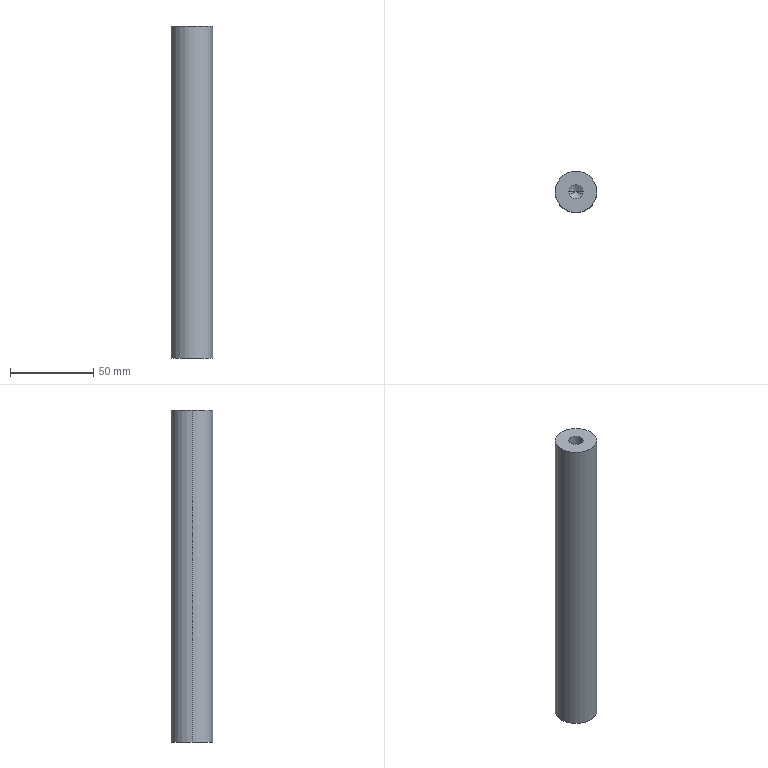Part | STEP file | B1-004 | 1 solid | 12 faces | box 25 x 25 x 200 mm | volume 96489 mm3 | cylinder 6 | cone 4 | plane 2 | commonest cylinder face diameters 8.5 x4 25 x2
STEP:
#1=CARTESIAN_POINT('',(0.,0.,0.));
#2=DIRECTION('',(0.,0.,1.));
#3=DIRECTION('',(1.,0.,0.));
#4=AXIS2_PLACEMENT_3D('',#1,#2,#3);
#5=CARTESIAN_POINT('',(4.25,0.,86.));
#6=VERTEX_POINT('',#5);
#7=CARTESIAN_POINT('',(4.25,0.,100.));
#8=VERTEX_POINT('',#7);
#9=CARTESIAN_POINT('',(4.25,0.,100.));
#10=DIRECTION('',(0.,0.,1.));
#11=VECTOR('',#10,1.);
#12=LINE('',#9,#11);
#13=CARTESIAN_POINT('',(0.,0.,100.));
#14=DIRECTION('',(0.,0.,1.));
#15=DIRECTION('',(1.,0.,0.));
#16=AXIS2_PLACEMENT_3D('',#13,#14,#15);
#17=CYLINDRICAL_SURFACE('',#16,4.25);
#18=CARTESIAN_POINT('',(6.283,0.));
#19=DIRECTION('',(0.,1.));
#20=VECTOR('',#19,1.);
#21=LINE('',#18,#20);
#22=(GEOMETRIC_REPRESENTATION_CONTEXT(2)PARAMETRIC_REPRESENTATION_CONTEXT()REPRESENTATION_CONTEXT('',''));
#23=DEFINITIONAL_REPRESENTATION('',(#21),#22);
#24=PCURVE('',#17,#23);
#25=CARTESIAN_POINT('',(0.,0.,100.));
#26=DIRECTION('',(0.,0.,1.));
#27=DIRECTION('',(1.,0.,0.));
#28=AXIS2_PLACEMENT_3D('',#25,#26,#27);
#29=CYLINDRICAL_SURFACE('',#28,4.25);
#30=CARTESIAN_POINT('',(0.,0.));
#31=DIRECTION('',(0.,1.));
#32=VECTOR('',#31,1.);
#33=LINE('',#30,#32);
#34=(GEOMETRIC_REPRESENTATION_CONTEXT(2)PARAMETRIC_REPRESENTATION_CONTEXT()REPRESENTATION_CONTEXT('',''));
#35=DEFINITIONAL_REPRESENTATION('',(#33),#34);
#36=PCURVE('',#29,#35);
#37=SURFACE_CURVE('',#12,(#24,#36),.PCURVE_S1.);
#38=EDGE_CURVE('',#6,#8,#37,.T.);
#39=ORIENTED_EDGE('',*,*,#38,.T.);
#40=CARTESIAN_POINT('',(-4.25,0.,100.));
#41=VERTEX_POINT('',#40);
#42=CARTESIAN_POINT('',(0.,0.,100.));
#43=DIRECTION('',(0.,0.,1.));
#44=DIRECTION('',(1.,0.,0.));
#45=AXIS2_PLACEMENT_3D('',#42,#43,#44);
#46=CIRCLE('',#45,4.25);
#47=CARTESIAN_POINT('',(0.,0.));
#48=DIRECTION('',(1.,0.));
#49=VECTOR('',#48,1.);
#50=LINE('',#47,#49);
#51=(GEOMETRIC_REPRESENTATION_CONTEXT(2)PARAMETRIC_REPRESENTATION_CONTEXT()REPRESENTATION_CONTEXT('',''));
#52=DEFINITIONAL_REPRESENTATION('',(#50),#51);
#53=PCURVE('',#17,#52);
#54=CARTESIAN_POINT('',(0.,0.,100.));
#55=DIRECTION('',(0.,0.,1.));
#56=DIRECTION('',(1.,0.,0.));
#57=AXIS2_PLACEMENT_3D('',#54,#55,#56);
#58=PLANE('',#57);
#59=CARTESIAN_POINT('',(0.,0.));
#60=DIRECTION('',(1.,0.));
#61=AXIS2_PLACEMENT_2D('',#59,#60);
#62=CIRCLE('',#61,4.25);
#63=(GEOMETRIC_REPRESENTATION_CONTEXT(2)PARAMETRIC_REPRESENTATION_CONTEXT()REPRESENTATION_CONTEXT('',''));
#64=DEFINITIONAL_REPRESENTATION('',(#62),#63);
#65=PCURVE('',#58,#64);
#66=SURFACE_CURVE('',#46,(#53,#65),.PCURVE_S1.);
#67=EDGE_CURVE('',#41,#8,#66,.T.);
#68=ORIENTED_EDGE('',*,*,#67,.F.);
#69=CARTESIAN_POINT('',(-4.25,0.,86.));
#70=VERTEX_POINT('',#69);
#71=CARTESIAN_POINT('',(-4.25,0.,100.));
#72=DIRECTION('',(0.,0.,1.));
#73=VECTOR('',#72,1.);
#74=LINE('',#71,#73);
#75=CARTESIAN_POINT('',(3.142,0.));
#76=DIRECTION('',(0.,1.));
#77=VECTOR('',#76,1.);
#78=LINE('',#75,#77);
#79=(GEOMETRIC_REPRESENTATION_CONTEXT(2)PARAMETRIC_REPRESENTATION_CONTEXT()REPRESENTATION_CONTEXT('',''));
#80=DEFINITIONAL_REPRESENTATION('',(#78),#79);
#81=PCURVE('',#17,#80);
#82=CARTESIAN_POINT('',(3.142,0.));
#83=DIRECTION('',(0.,1.));
#84=VECTOR('',#83,1.);
#85=LINE('',#82,#84);
#86=(GEOMETRIC_REPRESENTATION_CONTEXT(2)PARAMETRIC_REPRESENTATION_CONTEXT()REPRESENTATION_CONTEXT('',''));
#87=DEFINITIONAL_REPRESENTATION('',(#85),#86);
#88=PCURVE('',#29,#87);
#89=SURFACE_CURVE('',#74,(#81,#88),.PCURVE_S1.);
#90=EDGE_CURVE('',#70,#41,#89,.T.);
#91=ORIENTED_EDGE('',*,*,#90,.F.);
#92=CARTESIAN_POINT('',(0.,0.,86.));
#93=DIRECTION('',(0.,0.,1.));
#94=DIRECTION('',(1.,0.,0.));
#95=AXIS2_PLACEMENT_3D('',#92,#93,#94);
#96=CIRCLE('',#95,4.25);
#97=CARTESIAN_POINT('',(0.,-14.));
#98=DIRECTION('',(1.,0.));
#99=VECTOR('',#98,1.);
#100=LINE('',#97,#99);
#101=(GEOMETRIC_REPRESENTATION_CONTEXT(2)PARAMETRIC_REPRESENTATION_CONTEXT()REPRESENTATION_CONTEXT('',''));
#102=DEFINITIONAL_REPRESENTATION('',(#100),#101);
#103=PCURVE('',#17,#102);
#104=CARTESIAN_POINT('',(0.,0.,86.));
#105=DIRECTION('',(0.,0.,1.));
#106=DIRECTION('',(1.,0.,0.));
#107=AXIS2_PLACEMENT_3D('',#104,#105,#106);
#108=CONICAL_SURFACE('',#107,4.25,1.03);
#109=CARTESIAN_POINT('',(0.,0.));
#110=DIRECTION('',(1.,0.));
#111=VECTOR('',#110,1.);
#112=LINE('',#109,#111);
#113=(GEOMETRIC_REPRESENTATION_CONTEXT(2)PARAMETRIC_REPRESENTATION_CONTEXT()REPRESENTATION_CONTEXT('',''));
#114=DEFINITIONAL_REPRESENTATION('',(#112),#113);
#115=PCURVE('',#108,#114);
#116=SURFACE_CURVE('',#96,(#103,#115),.PCURVE_S1.);
#117=EDGE_CURVE('',#70,#6,#116,.T.);
#118=ORIENTED_EDGE('',*,*,#117,.T.);
#119=EDGE_LOOP('',(#39,#68,#91,#118));
#120=FACE_BOUND('',#119,.F.);
#121=ADVANCED_FACE('',(#120),#17,.F.);
#122=ORIENTED_EDGE('',*,*,#117,.F.);
#123=CARTESIAN_POINT('',(0.,0.,83.446));
#124=VERTEX_POINT('',#123);
#125=CARTESIAN_POINT('',(-4.25,0.,86.));
#126=DIRECTION('',(-0.8572,0.,0.515));
#127=VECTOR('',#126,1.);
#128=LINE('',#125,#127);
#129=CARTESIAN_POINT('',(3.142,-2.554));
#130=CARTESIAN_POINT('',(3.142,-2.515));
#131=CARTESIAN_POINT('',(3.142,-2.438));
#132=CARTESIAN_POINT('',(3.142,-2.322));
#133=CARTESIAN_POINT('',(3.142,-2.205));
#134=CARTESIAN_POINT('',(3.142,-2.089));
#135=CARTESIAN_POINT('',(3.142,-1.973));
#136=CARTESIAN_POINT('',(3.142,-1.857));
#137=CARTESIAN_POINT('',(3.142,-1.741));
#138=CARTESIAN_POINT('',(3.142,-1.625));
#139=CARTESIAN_POINT('',(3.142,-1.509));
#140=CARTESIAN_POINT('',(3.142,-1.393));
#141=CARTESIAN_POINT('',(3.142,-1.277));
#142=CARTESIAN_POINT('',(3.142,-1.161));
#143=CARTESIAN_POINT('',(3.142,-1.045));
#144=CARTESIAN_POINT('',(3.142,-0.9286));
#145=CARTESIAN_POINT('',(3.142,-0.8125));
#146=CARTESIAN_POINT('',(3.142,-0.6965));
#147=CARTESIAN_POINT('',(3.142,-0.5804));
#148=CARTESIAN_POINT('',(3.142,-0.4643));
#149=CARTESIAN_POINT('',(3.142,-0.3482));
#150=CARTESIAN_POINT('',(3.142,-0.2322));
#151=CARTESIAN_POINT('',(3.142,-0.1161));
#152=CARTESIAN_POINT('',(3.142,-0.03869));
#153=CARTESIAN_POINT('',(3.142,0.));
#154=B_SPLINE_CURVE_WITH_KNOTS('',3,(#129,#130,#131,#132,#133,#134,#135,#136,#137,#138,#139,#140,#141,#142,#143,#144,#145,#146,#147,#148,#149,#150,#151,#152,#153),.UNSPECIFIED.,.F.,.F.,(4,1,1,1,1,1,1,1,1,1,1,1,1,1,1,1,1,1,1,1,1,1,4),(-4.958,-4.733,-4.507,-4.282,-4.057,-3.831,-3.606,-3.381,-3.155,-2.93,-2.704,-2.479,-2.254,-2.028,-1.803,-1.578,-1.352,-1.127,-0.9015,-0.6761,-0.4507,-0.2254,0.),.UNSPECIFIED.);
#155=(GEOMETRIC_REPRESENTATION_CONTEXT(2)PARAMETRIC_REPRESENTATION_CONTEXT()REPRESENTATION_CONTEXT('',''));
#156=DEFINITIONAL_REPRESENTATION('',(#154),#155);
#157=PCURVE('',#108,#156);
#158=CARTESIAN_POINT('',(0.,0.,86.));
#159=DIRECTION('',(0.,0.,1.));
#160=DIRECTION('',(1.,0.,0.));
#161=AXIS2_PLACEMENT_3D('',#158,#159,#160);
#162=CONICAL_SURFACE('',#161,4.25,1.03);
#163=CARTESIAN_POINT('',(3.142,-2.554));
#164=CARTESIAN_POINT('',(3.142,-2.515));
#165=CARTESIAN_POINT('',(3.142,-2.438));
#166=CARTESIAN_POINT('',(3.142,-2.322));
#167=CARTESIAN_POINT('',(3.142,-2.205));
#168=CARTESIAN_POINT('',(3.142,-2.089));
#169=CARTESIAN_POINT('',(3.142,-1.973));
#170=CARTESIAN_POINT('',(3.142,-1.857));
#171=CARTESIAN_POINT('',(3.142,-1.741));
#172=CARTESIAN_POINT('',(3.142,-1.625));
#173=CARTESIAN_POINT('',(3.142,-1.509));
#174=CARTESIAN_POINT('',(3.142,-1.393));
#175=CARTESIAN_POINT('',(3.142,-1.277));
#176=CARTESIAN_POINT('',(3.142,-1.161));
#177=CARTESIAN_POINT('',(3.142,-1.045));
#178=CARTESIAN_POINT('',(3.142,-0.9286));
#179=CARTESIAN_POINT('',(3.142,-0.8125));
#180=CARTESIAN_POINT('',(3.142,-0.6965));
#181=CARTESIAN_POINT('',(3.142,-0.5804));
#182=CARTESIAN_POINT('',(3.142,-0.4643));
#183=CARTESIAN_POINT('',(3.142,-0.3482));
#184=CARTESIAN_POINT('',(3.142,-0.2322));
#185=CARTESIAN_POINT('',(3.142,-0.1161));
#186=CARTESIAN_POINT('',(3.142,-0.03869));
#187=CARTESIAN_POINT('',(3.142,0.));
#188=B_SPLINE_CURVE_WITH_KNOTS('',3,(#163,#164,#165,#166,#167,#168,#169,#170,#171,#172,#173,#174,#175,#176,#177,#178,#179,#180,#181,#182,#183,#184,#185,#186,#187),.UNSPECIFIED.,.F.,.F.,(4,1,1,1,1,1,1,1,1,1,1,1,1,1,1,1,1,1,1,1,1,1,4),(-4.958,-4.733,-4.507,-4.282,-4.057,-3.831,-3.606,-3.381,-3.155,-2.93,-2.704,-2.479,-2.254,-2.028,-1.803,-1.578,-1.352,-1.127,-0.9015,-0.6761,-0.4507,-0.2254,0.),.UNSPECIFIED.);
#189=(GEOMETRIC_REPRESENTATION_CONTEXT(2)PARAMETRIC_REPRESENTATION_CONTEXT()REPRESENTATION_CONTEXT('',''));
#190=DEFINITIONAL_REPRESENTATION('',(#188),#189);
#191=PCURVE('',#162,#190);
#192=SURFACE_CURVE('',#128,(#157,#191),.PCURVE_S1.);
#193=EDGE_CURVE('',#124,#70,#192,.T.);
#194=ORIENTED_EDGE('',*,*,#193,.F.);
#195=CARTESIAN_POINT('',(4.25,0.,86.));
#196=DIRECTION('',(0.8572,0.,0.515));
#197=VECTOR('',#196,1.);
#198=LINE('',#195,#197);
#199=CARTESIAN_POINT('',(6.283,0.));
#200=DIRECTION('',(0.,1.));
#201=VECTOR('',#200,1.);
#202=LINE('',#199,#201);
#203=(GEOMETRIC_REPRESENTATION_CONTEXT(2)PARAMETRIC_REPRESENTATION_CONTEXT()REPRESENTATION_CONTEXT('',''));
#204=DEFINITIONAL_REPRESENTATION('',(#202),#203);
#205=PCURVE('',#108,#204);
#206=CARTESIAN_POINT('',(0.,0.));
#207=DIRECTION('',(0.,1.));
#208=VECTOR('',#207,1.);
#209=LINE('',#206,#208);
#210=(GEOMETRIC_REPRESENTATION_CONTEXT(2)PARAMETRIC_REPRESENTATION_CONTEXT()REPRESENTATION_CONTEXT('',''));
#211=DEFINITIONAL_REPRESENTATION('',(#209),#210);
#212=PCURVE('',#162,#211);
#213=SURFACE_CURVE('',#198,(#205,#212),.PCURVE_S1.);
#214=EDGE_CURVE('',#124,#6,#213,.T.);
#215=ORIENTED_EDGE('',*,*,#214,.T.);
#216=EDGE_LOOP('',(#122,#194,#215));
#217=FACE_BOUND('',#216,.F.);
#218=ADVANCED_FACE('',(#217),#108,.F.);
#219=CARTESIAN_POINT('',(-4.25,0.,-86.));
#220=VERTEX_POINT('',#219);
#221=CARTESIAN_POINT('',(-4.25,0.,-100.));
#222=VERTEX_POINT('',#221);
#223=CARTESIAN_POINT('',(-4.25,0.,-100.));
#224=DIRECTION('',(0.,0.,-1.));
#225=VECTOR('',#224,1.);
#226=LINE('',#223,#225);
#227=CARTESIAN_POINT('',(0.,0.,-100.));
#228=DIRECTION('',(0.,0.,-1.));
#229=DIRECTION('',(-1.,0.,0.));
#230=AXIS2_PLACEMENT_3D('',#227,#228,#229);
#231=CYLINDRICAL_SURFACE('',#230,4.25);
#232=CARTESIAN_POINT('',(6.283,0.));
#233=DIRECTION('',(0.,1.));
#234=VECTOR('',#233,1.);
#235=LINE('',#232,#234);
#236=(GEOMETRIC_REPRESENTATION_CONTEXT(2)PARAMETRIC_REPRESENTATION_CONTEXT()REPRESENTATION_CONTEXT('',''));
#237=DEFINITIONAL_REPRESENTATION('',(#235),#236);
#238=PCURVE('',#231,#237);
#239=CARTESIAN_POINT('',(0.,0.,-100.));
#240=DIRECTION('',(0.,0.,-1.));
#241=DIRECTION('',(-1.,0.,0.));
#242=AXIS2_PLACEMENT_3D('',#239,#240,#241);
#243=CYLINDRICAL_SURFACE('',#242,4.25);
#244=CARTESIAN_POINT('',(0.,0.));
#245=DIRECTION('',(0.,1.));
#246=VECTOR('',#245,1.);
#247=LINE('',#244,#246);
#248=(GEOMETRIC_REPRESENTATION_CONTEXT(2)PARAMETRIC_REPRESENTATION_CONTEXT()REPRESENTATION_CONTEXT('',''));
#249=DEFINITIONAL_REPRESENTATION('',(#247),#248);
#250=PCURVE('',#243,#249);
#251=SURFACE_CURVE('',#226,(#238,#250),.PCURVE_S1.);
#252=EDGE_CURVE('',#220,#222,#251,.T.);
#253=ORIENTED_EDGE('',*,*,#252,.T.);
#254=CARTESIAN_POINT('',(4.25,0.,-100.));
#255=VERTEX_POINT('',#254);
#256=CARTESIAN_POINT('',(0.,0.,-100.));
#257=DIRECTION('',(0.,0.,-1.));
#258=DIRECTION('',(-1.,0.,0.));
#259=AXIS2_PLACEMENT_3D('',#256,#257,#258);
#260=CIRCLE('',#259,4.25);
#261=CARTESIAN_POINT('',(0.,0.));
#262=DIRECTION('',(1.,0.));
#263=VECTOR('',#262,1.);
#264=LINE('',#261,#263);
#265=(GEOMETRIC_REPRESENTATION_CONTEXT(2)PARAMETRIC_REPRESENTATION_CONTEXT()REPRESENTATION_CONTEXT('',''));
#266=DEFINITIONAL_REPRESENTATION('',(#264),#265);
#267=PCURVE('',#231,#266);
#268=CARTESIAN_POINT('',(0.,0.,-100.));
#269=DIRECTION('',(0.,0.,1.));
#270=DIRECTION('',(1.,0.,0.));
#271=AXIS2_PLACEMENT_3D('',#268,#269,#270);
#272=PLANE('',#271);
#273=CARTESIAN_POINT('',(-4.25,0.));
#274=CARTESIAN_POINT('',(-4.25,7.361));
#275=CARTESIAN_POINT('',(2.125,3.681));
#276=CARTESIAN_POINT('',(8.5,0.));
#277=CARTESIAN_POINT('',(2.125,-3.681));
#278=CARTESIAN_POINT('',(-4.25,-7.361));
#279=CARTESIAN_POINT('',(-4.25,0.));
#280=(BOUNDED_CURVE()B_SPLINE_CURVE(2,(#273,#274,#275,#276,#277,#278,#279),.UNSPECIFIED.,.T.,.F.)B_SPLINE_CURVE_WITH_KNOTS((1,2,2,2,2,1),(-2.094,0.,2.094,4.189,6.283,8.378),.UNSPECIFIED.)CURVE()GEOMETRIC_REPRESENTATION_ITEM()RATIONAL_B_SPLINE_CURVE((1.,0.5,1.,0.5,1.,0.5,1.))REPRESENTATION_ITEM(''));
#281=(GEOMETRIC_REPRESENTATION_CONTEXT(2)PARAMETRIC_REPRESENTATION_CONTEXT()REPRESENTATION_CONTEXT('',''));
#282=DEFINITIONAL_REPRESENTATION('',(#280),#281);
#283=PCURVE('',#272,#282);
#284=SURFACE_CURVE('',#260,(#267,#283),.PCURVE_S1.);
#285=EDGE_CURVE('',#255,#222,#284,.T.);
#286=ORIENTED_EDGE('',*,*,#285,.F.);
#287=CARTESIAN_POINT('',(4.25,0.,-86.));
#288=VERTEX_POINT('',#287);
#289=CARTESIAN_POINT('',(4.25,0.,-100.));
#290=DIRECTION('',(0.,0.,-1.));
#291=VECTOR('',#290,1.);
#292=LINE('',#289,#291);
#293=CARTESIAN_POINT('',(3.142,0.));
#294=DIRECTION('',(0.,1.));
#295=VECTOR('',#294,1.);
#296=LINE('',#293,#295);
#297=(GEOMETRIC_REPRESENTATION_CONTEXT(2)PARAMETRIC_REPRESENTATION_CONTEXT()REPRESENTATION_CONTEXT('',''));
#298=DEFINITIONAL_REPRESENTATION('',(#296),#297);
#299=PCURVE('',#231,#298);
#300=CARTESIAN_POINT('',(3.142,0.));
#301=DIRECTION('',(0.,1.));
#302=VECTOR('',#301,1.);
#303=LINE('',#300,#302);
#304=(GEOMETRIC_REPRESENTATION_CONTEXT(2)PARAMETRIC_REPRESENTATION_CONTEXT()REPRESENTATION_CONTEXT('',''));
#305=DEFINITIONAL_REPRESENTATION('',(#303),#304);
#306=PCURVE('',#243,#305);
#307=SURFACE_CURVE('',#292,(#299,#306),.PCURVE_S1.);
#308=EDGE_CURVE('',#288,#255,#307,.T.);
#309=ORIENTED_EDGE('',*,*,#308,.F.);
#310=CARTESIAN_POINT('',(0.,0.,-86.));
#311=DIRECTION('',(0.,0.,-1.));
#312=DIRECTION('',(-1.,0.,0.));
#313=AXIS2_PLACEMENT_3D('',#310,#311,#312);
#314=CIRCLE('',#313,4.25);
#315=CARTESIAN_POINT('',(0.,-14.));
#316=DIRECTION('',(1.,0.));
#317=VECTOR('',#316,1.);
#318=LINE('',#315,#317);
#319=(GEOMETRIC_REPRESENTATION_CONTEXT(2)PARAMETRIC_REPRESENTATION_CONTEXT()REPRESENTATION_CONTEXT('',''));
#320=DEFINITIONAL_REPRESENTATION('',(#318),#319);
#321=PCURVE('',#231,#320);
#322=CARTESIAN_POINT('',(0.,0.,-86.));
#323=DIRECTION('',(0.,0.,-1.));
#324=DIRECTION('',(-1.,0.,0.));
#325=AXIS2_PLACEMENT_3D('',#322,#323,#324);
#326=CONICAL_SURFACE('',#325,4.25,1.03);
#327=CARTESIAN_POINT('',(0.,0.));
#328=DIRECTION('',(1.,0.));
#329=VECTOR('',#328,1.);
#330=LINE('',#327,#329);
#331=(GEOMETRIC_REPRESENTATION_CONTEXT(2)PARAMETRIC_REPRESENTATION_CONTEXT()REPRESENTATION_CONTEXT('',''));
#332=DEFINITIONAL_REPRESENTATION('',(#330),#331);
#333=PCURVE('',#326,#332);
#334=SURFACE_CURVE('',#314,(#321,#333),.PCURVE_S1.);
#335=EDGE_CURVE('',#288,#220,#334,.T.);
#336=ORIENTED_EDGE('',*,*,#335,.T.);
#337=EDGE_LOOP('',(#253,#286,#309,#336));
#338=FACE_BOUND('',#337,.F.);
#339=ADVANCED_FACE('',(#338),#231,.F.);
#340=ORIENTED_EDGE('',*,*,#335,.F.);
#341=CARTESIAN_POINT('',(0.,0.,-83.446));
#342=VERTEX_POINT('',#341);
#343=CARTESIAN_POINT('',(4.25,0.,-86.));
#344=DIRECTION('',(0.8572,0.,-0.515));
#345=VECTOR('',#344,1.);
#346=LINE('',#343,#345);
#347=CARTESIAN_POINT('',(3.142,0.));
#348=DIRECTION('',(0.,1.));
#349=VECTOR('',#348,1.);
#350=LINE('',#347,#349);
#351=(GEOMETRIC_REPRESENTATION_CONTEXT(2)PARAMETRIC_REPRESENTATION_CONTEXT()REPRESENTATION_CONTEXT('',''));
#352=DEFINITIONAL_REPRESENTATION('',(#350),#351);
#353=PCURVE('',#326,#352);
#354=CARTESIAN_POINT('',(0.,0.,-86.));
#355=DIRECTION('',(0.,0.,-1.));
#356=DIRECTION('',(-1.,0.,0.));
#357=AXIS2_PLACEMENT_3D('',#354,#355,#356);
#358=CONICAL_SURFACE('',#357,4.25,1.03);
#359=CARTESIAN_POINT('',(3.142,0.));
#360=DIRECTION('',(0.,1.));
#361=VECTOR('',#360,1.);
#362=LINE('',#359,#361);
#363=(GEOMETRIC_REPRESENTATION_CONTEXT(2)PARAMETRIC_REPRESENTATION_CONTEXT()REPRESENTATION_CONTEXT('',''));
#364=DEFINITIONAL_REPRESENTATION('',(#362),#363);
#365=PCURVE('',#358,#364);
#366=SURFACE_CURVE('',#346,(#353,#365),.PCURVE_S1.);
#367=EDGE_CURVE('',#342,#288,#366,.T.);
#368=ORIENTED_EDGE('',*,*,#367,.F.);
#369=CARTESIAN_POINT('',(-4.25,0.,-86.));
#370=DIRECTION('',(-0.8572,0.,-0.515));
#371=VECTOR('',#370,1.);
#372=LINE('',#369,#371);
#373=CARTESIAN_POINT('',(6.283,-2.554));
#374=CARTESIAN_POINT('',(6.283,-2.515));
#375=CARTESIAN_POINT('',(6.283,-2.438));
#376=CARTESIAN_POINT('',(6.283,-2.322));
#377=CARTESIAN_POINT('',(6.283,-2.205));
#378=CARTESIAN_POINT('',(6.283,-2.089));
#379=CARTESIAN_POINT('',(6.283,-1.973));
#380=CARTESIAN_POINT('',(6.283,-1.857));
#381=CARTESIAN_POINT('',(6.283,-1.741));
#382=CARTESIAN_POINT('',(6.283,-1.625));
#383=CARTESIAN_POINT('',(6.283,-1.509));
#384=CARTESIAN_POINT('',(6.283,-1.393));
#385=CARTESIAN_POINT('',(6.283,-1.277));
#386=CARTESIAN_POINT('',(6.283,-1.161));
#387=CARTESIAN_POINT('',(6.283,-1.045));
#388=CARTESIAN_POINT('',(6.283,-0.9286));
#389=CARTESIAN_POINT('',(6.283,-0.8125));
#390=CARTESIAN_POINT('',(6.283,-0.6965));
#391=CARTESIAN_POINT('',(6.283,-0.5804));
#392=CARTESIAN_POINT('',(6.283,-0.4643));
#393=CARTESIAN_POINT('',(6.283,-0.3482));
#394=CARTESIAN_POINT('',(6.283,-0.2322));
#395=CARTESIAN_POINT('',(6.283,-0.1161));
#396=CARTESIAN_POINT('',(6.283,-0.03869));
#397=CARTESIAN_POINT('',(6.283,0.));
#398=B_SPLINE_CURVE_WITH_KNOTS('',3,(#373,#374,#375,#376,#377,#378,#379,#380,#381,#382,#383,#384,#385,#386,#387,#388,#389,#390,#391,#392,#393,#394,#395,#396,#397),.UNSPECIFIED.,.F.,.F.,(4,1,1,1,1,1,1,1,1,1,1,1,1,1,1,1,1,1,1,1,1,1,4),(-4.958,-4.733,-4.507,-4.282,-4.057,-3.831,-3.606,-3.381,-3.155,-2.93,-2.704,-2.479,-2.254,-2.028,-1.803,-1.578,-1.352,-1.127,-0.9015,-0.6761,-0.4507,-0.2254,0.),.UNSPECIFIED.);
#399=(GEOMETRIC_REPRESENTATION_CONTEXT(2)PARAMETRIC_REPRESENTATION_CONTEXT()REPRESENTATION_CONTEXT('',''));
#400=DEFINITIONAL_REPRESENTATION('',(#398),#399);
#401=PCURVE('',#326,#400);
#402=CARTESIAN_POINT('',(0.,-2.554));
#403=CARTESIAN_POINT('',(0.,-2.515));
#404=CARTESIAN_POINT('',(0.,-2.438));
#405=CARTESIAN_POINT('',(0.,-2.322));
#406=CARTESIAN_POINT('',(0.,-2.205));
#407=CARTESIAN_POINT('',(0.,-2.089));
#408=CARTESIAN_POINT('',(0.,-1.973));
#409=CARTESIAN_POINT('',(0.,-1.857));
#410=CARTESIAN_POINT('',(0.,-1.741));
#411=CARTESIAN_POINT('',(0.,-1.625));
#412=CARTESIAN_POINT('',(0.,-1.509));
#413=CARTESIAN_POINT('',(0.,-1.393));
#414=CARTESIAN_POINT('',(0.,-1.277));
#415=CARTESIAN_POINT('',(0.,-1.161));
#416=CARTESIAN_POINT('',(0.,-1.045));
#417=CARTESIAN_POINT('',(0.,-0.9286));
#418=CARTESIAN_POINT('',(0.,-0.8125));
#419=CARTESIAN_POINT('',(0.,-0.6965));
#420=CARTESIAN_POINT('',(0.,-0.5804));
#421=CARTESIAN_POINT('',(0.,-0.4643));
#422=CARTESIAN_POINT('',(0.,-0.3482));
#423=CARTESIAN_POINT('',(0.,-0.2322));
#424=CARTESIAN_POINT('',(0.,-0.1161));
#425=CARTESIAN_POINT('',(0.,-0.03869));
#426=CARTESIAN_POINT('',(0.,0.));
#427=B_SPLINE_CURVE_WITH_KNOTS('',3,(#402,#403,#404,#405,#406,#407,#408,#409,#410,#411,#412,#413,#414,#415,#416,#417,#418,#419,#420,#421,#422,#423,#424,#425,#426),.UNSPECIFIED.,.F.,.F.,(4,1,1,1,1,1,1,1,1,1,1,1,1,1,1,1,1,1,1,1,1,1,4),(-4.958,-4.733,-4.507,-4.282,-4.057,-3.831,-3.606,-3.381,-3.155,-2.93,-2.704,-2.479,-2.254,-2.028,-1.803,-1.578,-1.352,-1.127,-0.9015,-0.6761,-0.4507,-0.2254,0.),.UNSPECIFIED.);
#428=(GEOMETRIC_REPRESENTATION_CONTEXT(2)PARAMETRIC_REPRESENTATION_CONTEXT()REPRESENTATION_CONTEXT('',''));
#429=DEFINITIONAL_REPRESENTATION('',(#427),#428);
#430=PCURVE('',#358,#429);
#431=SURFACE_CURVE('',#372,(#401,#430),.PCURVE_S1.);
#432=EDGE_CURVE('',#342,#220,#431,.T.);
#433=ORIENTED_EDGE('',*,*,#432,.T.);
#434=EDGE_LOOP('',(#340,#368,#433));
#435=FACE_BOUND('',#434,.F.);
#436=ADVANCED_FACE('',(#435),#326,.F.);
#437=CARTESIAN_POINT('',(12.5,0.,100.));
#438=VERTEX_POINT('',#437);
#439=CARTESIAN_POINT('',(-12.5,0.,100.));
#440=VERTEX_POINT('',#439);
#441=CARTESIAN_POINT('',(0.,0.,100.));
#442=DIRECTION('',(0.,0.,1.));
#443=DIRECTION('',(1.,0.,0.));
#444=AXIS2_PLACEMENT_3D('',#441,#442,#443);
#445=CIRCLE('',#444,12.5);
#446=CARTESIAN_POINT('',(0.,0.,100.));
#447=DIRECTION('',(0.,0.,-1.));
#448=DIRECTION('',(-1.,0.,0.));
#449=AXIS2_PLACEMENT_3D('',#446,#447,#448);
#450=CYLINDRICAL_SURFACE('',#449,12.5);
#451=CARTESIAN_POINT('',(3.142,0.));
#452=DIRECTION('',(-1.,0.));
#453=VECTOR('',#452,1.);
#454=LINE('',#451,#453);
#455=(GEOMETRIC_REPRESENTATION_CONTEXT(2)PARAMETRIC_REPRESENTATION_CONTEXT()REPRESENTATION_CONTEXT('',''));
#456=DEFINITIONAL_REPRESENTATION('',(#454),#455);
#457=PCURVE('',#450,#456);
#458=CARTESIAN_POINT('',(0.,0.));
#459=DIRECTION('',(1.,0.));
#460=AXIS2_PLACEMENT_2D('',#458,#459);
#461=CIRCLE('',#460,12.5);
#462=(GEOMETRIC_REPRESENTATION_CONTEXT(2)PARAMETRIC_REPRESENTATION_CONTEXT()REPRESENTATION_CONTEXT('',''));
#463=DEFINITIONAL_REPRESENTATION('',(#461),#462);
#464=PCURVE('',#58,#463);
#465=SURFACE_CURVE('',#445,(#457,#464),.PCURVE_S1.);
#466=EDGE_CURVE('',#438,#440,#465,.T.);
#467=ORIENTED_EDGE('',*,*,#466,.F.);
#468=CARTESIAN_POINT('',(12.5,0.,-100.));
#469=VERTEX_POINT('',#468);
#470=CARTESIAN_POINT('',(12.5,0.,100.));
#471=DIRECTION('',(0.,0.,-1.));
#472=VECTOR('',#471,1.);
#473=LINE('',#470,#472);
#474=CARTESIAN_POINT('',(3.142,0.));
#475=DIRECTION('',(0.,1.));
#476=VECTOR('',#475,1.);
#477=LINE('',#474,#476);
#478=(GEOMETRIC_REPRESENTATION_CONTEXT(2)PARAMETRIC_REPRESENTATION_CONTEXT()REPRESENTATION_CONTEXT('',''));
#479=DEFINITIONAL_REPRESENTATION('',(#477),#478);
#480=PCURVE('',#450,#479);
#481=CARTESIAN_POINT('',(0.,0.,100.));
#482=DIRECTION('',(0.,0.,-1.));
#483=DIRECTION('',(-1.,0.,0.));
#484=AXIS2_PLACEMENT_3D('',#481,#482,#483);
#485=CYLINDRICAL_SURFACE('',#484,12.5);
#486=CARTESIAN_POINT('',(3.142,0.));
#487=DIRECTION('',(0.,1.));
#488=VECTOR('',#487,1.);
#489=LINE('',#486,#488);
#490=(GEOMETRIC_REPRESENTATION_CONTEXT(2)PARAMETRIC_REPRESENTATION_CONTEXT()REPRESENTATION_CONTEXT('',''));
#491=DEFINITIONAL_REPRESENTATION('',(#489),#490);
#492=PCURVE('',#485,#491);
#493=SURFACE_CURVE('',#473,(#480,#492),.PCURVE_S1.);
#494=EDGE_CURVE('',#438,#469,#493,.T.);
#495=ORIENTED_EDGE('',*,*,#494,.T.);
#496=CARTESIAN_POINT('',(-12.5,0.,-100.));
#497=VERTEX_POINT('',#496);
#498=CARTESIAN_POINT('',(0.,0.,-100.));
#499=DIRECTION('',(0.,0.,1.));
#500=DIRECTION('',(1.,0.,0.));
#501=AXIS2_PLACEMENT_3D('',#498,#499,#500);
#502=CIRCLE('',#501,12.5);
#503=CARTESIAN_POINT('',(3.142,200.));
#504=DIRECTION('',(-1.,0.));
#505=VECTOR('',#504,1.);
#506=LINE('',#503,#505);
#507=(GEOMETRIC_REPRESENTATION_CONTEXT(2)PARAMETRIC_REPRESENTATION_CONTEXT()REPRESENTATION_CONTEXT('',''));
#508=DEFINITIONAL_REPRESENTATION('',(#506),#507);
#509=PCURVE('',#450,#508);
#510=CARTESIAN_POINT('',(0.,0.));
#511=DIRECTION('',(1.,0.));
#512=AXIS2_PLACEMENT_2D('',#510,#511);
#513=CIRCLE('',#512,12.5);
#514=(GEOMETRIC_REPRESENTATION_CONTEXT(2)PARAMETRIC_REPRESENTATION_CONTEXT()REPRESENTATION_CONTEXT('',''));
#515=DEFINITIONAL_REPRESENTATION('',(#513),#514);
#516=PCURVE('',#272,#515);
#517=SURFACE_CURVE('',#502,(#509,#516),.PCURVE_S1.);
#518=EDGE_CURVE('',#469,#497,#517,.T.);
#519=ORIENTED_EDGE('',*,*,#518,.T.);
#520=CARTESIAN_POINT('',(-12.5,0.,100.));
#521=DIRECTION('',(0.,0.,-1.));
#522=VECTOR('',#521,1.);
#523=LINE('',#520,#522);
#524=CARTESIAN_POINT('',(0.,0.));
#525=DIRECTION('',(0.,1.));
#526=VECTOR('',#525,1.);
#527=LINE('',#524,#526);
#528=(GEOMETRIC_REPRESENTATION_CONTEXT(2)PARAMETRIC_REPRESENTATION_CONTEXT()REPRESENTATION_CONTEXT('',''));
#529=DEFINITIONAL_REPRESENTATION('',(#527),#528);
#530=PCURVE('',#450,#529);
#531=CARTESIAN_POINT('',(6.283,0.));
#532=DIRECTION('',(0.,1.));
#533=VECTOR('',#532,1.);
#534=LINE('',#531,#533);
#535=(GEOMETRIC_REPRESENTATION_CONTEXT(2)PARAMETRIC_REPRESENTATION_CONTEXT()REPRESENTATION_CONTEXT('',''));
#536=DEFINITIONAL_REPRESENTATION('',(#534),#535);
#537=PCURVE('',#485,#536);
#538=SURFACE_CURVE('',#523,(#530,#537),.PCURVE_S1.);
#539=EDGE_CURVE('',#440,#497,#538,.T.);
#540=ORIENTED_EDGE('',*,*,#539,.F.);
#541=EDGE_LOOP('',(#467,#495,#519,#540));
#542=FACE_BOUND('',#541,.T.);
#543=ADVANCED_FACE('',(#542),#450,.T.);
#544=ORIENTED_EDGE('',*,*,#494,.F.);
#545=CARTESIAN_POINT('',(0.,0.,100.));
#546=DIRECTION('',(0.,0.,1.));
#547=DIRECTION('',(1.,0.,0.));
#548=AXIS2_PLACEMENT_3D('',#545,#546,#547);
#549=CIRCLE('',#548,12.5);
#550=CARTESIAN_POINT('',(9.425,0.));
#551=DIRECTION('',(-1.,0.));
#552=VECTOR('',#551,1.);
#553=LINE('',#550,#552);
#554=(GEOMETRIC_REPRESENTATION_CONTEXT(2)PARAMETRIC_REPRESENTATION_CONTEXT()REPRESENTATION_CONTEXT('',''));
#555=DEFINITIONAL_REPRESENTATION('',(#553),#554);
#556=PCURVE('',#485,#555);
#557=CARTESIAN_POINT('',(0.,0.));
#558=DIRECTION('',(1.,0.));
#559=AXIS2_PLACEMENT_2D('',#557,#558);
#560=CIRCLE('',#559,12.5);
#561=(GEOMETRIC_REPRESENTATION_CONTEXT(2)PARAMETRIC_REPRESENTATION_CONTEXT()REPRESENTATION_CONTEXT('',''));
#562=DEFINITIONAL_REPRESENTATION('',(#560),#561);
#563=PCURVE('',#58,#562);
#564=SURFACE_CURVE('',#549,(#556,#563),.PCURVE_S1.);
#565=EDGE_CURVE('',#440,#438,#564,.T.);
#566=ORIENTED_EDGE('',*,*,#565,.F.);
#567=ORIENTED_EDGE('',*,*,#539,.T.);
#568=CARTESIAN_POINT('',(0.,0.,-100.));
#569=DIRECTION('',(0.,0.,1.));
#570=DIRECTION('',(1.,0.,0.));
#571=AXIS2_PLACEMENT_3D('',#568,#569,#570);
#572=CIRCLE('',#571,12.5);
#573=CARTESIAN_POINT('',(9.425,200.));
#574=DIRECTION('',(-1.,0.));
#575=VECTOR('',#574,1.);
#576=LINE('',#573,#575);
#577=(GEOMETRIC_REPRESENTATION_CONTEXT(2)PARAMETRIC_REPRESENTATION_CONTEXT()REPRESENTATION_CONTEXT('',''));
#578=DEFINITIONAL_REPRESENTATION('',(#576),#577);
#579=PCURVE('',#485,#578);
#580=CARTESIAN_POINT('',(0.,0.));
#581=DIRECTION('',(1.,0.));
#582=AXIS2_PLACEMENT_2D('',#580,#581);
#583=CIRCLE('',#582,12.5);
#584=(GEOMETRIC_REPRESENTATION_CONTEXT(2)PARAMETRIC_REPRESENTATION_CONTEXT()REPRESENTATION_CONTEXT('',''));
#585=DEFINITIONAL_REPRESENTATION('',(#583),#584);
#586=PCURVE('',#272,#585);
#587=SURFACE_CURVE('',#572,(#579,#586),.PCURVE_S1.);
#588=EDGE_CURVE('',#497,#469,#587,.T.);
#589=ORIENTED_EDGE('',*,*,#588,.T.);
#590=EDGE_LOOP('',(#544,#566,#567,#589));
#591=FACE_BOUND('',#590,.T.);
#592=ADVANCED_FACE('',(#591),#485,.T.);
#593=CARTESIAN_POINT('',(0.,0.,100.));
#594=DIRECTION('',(0.,0.,1.));
#595=DIRECTION('',(1.,0.,0.));
#596=AXIS2_PLACEMENT_3D('',#593,#594,#595);
#597=CIRCLE('',#596,4.25);
#598=CARTESIAN_POINT('',(0.,0.));
#599=DIRECTION('',(1.,0.));
#600=AXIS2_PLACEMENT_2D('',#598,#599);
#601=CIRCLE('',#600,4.25);
#602=(GEOMETRIC_REPRESENTATION_CONTEXT(2)PARAMETRIC_REPRESENTATION_CONTEXT()REPRESENTATION_CONTEXT('',''));
#603=DEFINITIONAL_REPRESENTATION('',(#601),#602);
#604=PCURVE('',#58,#603);
#605=CARTESIAN_POINT('',(0.,0.));
#606=DIRECTION('',(1.,0.));
#607=VECTOR('',#606,1.);
#608=LINE('',#605,#607);
#609=(GEOMETRIC_REPRESENTATION_CONTEXT(2)PARAMETRIC_REPRESENTATION_CONTEXT()REPRESENTATION_CONTEXT('',''));
#610=DEFINITIONAL_REPRESENTATION('',(#608),#609);
#611=PCURVE('',#29,#610);
#612=SURFACE_CURVE('',#597,(#604,#611),.PCURVE_S1.);
#613=EDGE_CURVE('',#8,#41,#612,.T.);
#614=ORIENTED_EDGE('',*,*,#613,.F.);
#615=ORIENTED_EDGE('',*,*,#67,.F.);
#616=EDGE_LOOP('',(#614,#615));
#617=FACE_BOUND('',#616,.T.);
#618=ORIENTED_EDGE('',*,*,#565,.T.);
#619=ORIENTED_EDGE('',*,*,#466,.T.);
#620=EDGE_LOOP('',(#618,#619));
#621=FACE_BOUND('',#620,.T.);
#622=ADVANCED_FACE('',(#617,#621),#58,.T.);
#623=CARTESIAN_POINT('',(0.,0.,-100.));
#624=DIRECTION('',(0.,0.,-1.));
#625=DIRECTION('',(-1.,0.,0.));
#626=AXIS2_PLACEMENT_3D('',#623,#624,#625);
#627=CIRCLE('',#626,4.25);
#628=CARTESIAN_POINT('',(-4.25,0.));
#629=CARTESIAN_POINT('',(-4.25,7.361));
#630=CARTESIAN_POINT('',(2.125,3.681));
#631=CARTESIAN_POINT('',(8.5,0.));
#632=CARTESIAN_POINT('',(2.125,-3.681));
#633=CARTESIAN_POINT('',(-4.25,-7.361));
#634=CARTESIAN_POINT('',(-4.25,0.));
#635=(BOUNDED_CURVE()B_SPLINE_CURVE(2,(#628,#629,#630,#631,#632,#633,#634),.UNSPECIFIED.,.T.,.F.)B_SPLINE_CURVE_WITH_KNOTS((1,2,2,2,2,1),(-2.094,0.,2.094,4.189,6.283,8.378),.UNSPECIFIED.)CURVE()GEOMETRIC_REPRESENTATION_ITEM()RATIONAL_B_SPLINE_CURVE((1.,0.5,1.,0.5,1.,0.5,1.))REPRESENTATION_ITEM(''));
#636=(GEOMETRIC_REPRESENTATION_CONTEXT(2)PARAMETRIC_REPRESENTATION_CONTEXT()REPRESENTATION_CONTEXT('',''));
#637=DEFINITIONAL_REPRESENTATION('',(#635),#636);
#638=PCURVE('',#272,#637);
#639=CARTESIAN_POINT('',(0.,0.));
#640=DIRECTION('',(1.,0.));
#641=VECTOR('',#640,1.);
#642=LINE('',#639,#641);
#643=(GEOMETRIC_REPRESENTATION_CONTEXT(2)PARAMETRIC_REPRESENTATION_CONTEXT()REPRESENTATION_CONTEXT('',''));
#644=DEFINITIONAL_REPRESENTATION('',(#642),#643);
#645=PCURVE('',#243,#644);
#646=SURFACE_CURVE('',#627,(#638,#645),.PCURVE_S1.);
#647=EDGE_CURVE('',#222,#255,#646,.T.);
#648=ORIENTED_EDGE('',*,*,#647,.F.);
#649=ORIENTED_EDGE('',*,*,#285,.F.);
#650=EDGE_LOOP('',(#648,#649));
#651=FACE_BOUND('',#650,.T.);
#652=ORIENTED_EDGE('',*,*,#588,.F.);
#653=ORIENTED_EDGE('',*,*,#518,.F.);
#654=EDGE_LOOP('',(#652,#653));
#655=FACE_BOUND('',#654,.T.);
#656=ADVANCED_FACE('',(#651,#655),#272,.F.);
#657=CARTESIAN_POINT('',(0.,0.,-86.));
#658=DIRECTION('',(0.,0.,-1.));
#659=DIRECTION('',(-1.,0.,0.));
#660=AXIS2_PLACEMENT_3D('',#657,#658,#659);
#661=CIRCLE('',#660,4.25);
#662=CARTESIAN_POINT('',(0.,0.));
#663=DIRECTION('',(1.,0.));
#664=VECTOR('',#663,1.);
#665=LINE('',#662,#664);
#666=(GEOMETRIC_REPRESENTATION_CONTEXT(2)PARAMETRIC_REPRESENTATION_CONTEXT()REPRESENTATION_CONTEXT('',''));
#667=DEFINITIONAL_REPRESENTATION('',(#665),#666);
#668=PCURVE('',#358,#667);
#669=CARTESIAN_POINT('',(0.,-14.));
#670=DIRECTION('',(1.,0.));
#671=VECTOR('',#670,1.);
#672=LINE('',#669,#671);
#673=(GEOMETRIC_REPRESENTATION_CONTEXT(2)PARAMETRIC_REPRESENTATION_CONTEXT()REPRESENTATION_CONTEXT('',''));
#674=DEFINITIONAL_REPRESENTATION('',(#672),#673);
#675=PCURVE('',#243,#674);
#676=SURFACE_CURVE('',#661,(#668,#675),.PCURVE_S1.);
#677=EDGE_CURVE('',#220,#288,#676,.T.);
#678=ORIENTED_EDGE('',*,*,#677,.F.);
#679=ORIENTED_EDGE('',*,*,#432,.F.);
#680=ORIENTED_EDGE('',*,*,#367,.T.);
#681=EDGE_LOOP('',(#678,#679,#680));
#682=FACE_BOUND('',#681,.F.);
#683=ADVANCED_FACE('',(#682),#358,.F.);
#684=ORIENTED_EDGE('',*,*,#647,.F.);
#685=ORIENTED_EDGE('',*,*,#252,.F.);
#686=ORIENTED_EDGE('',*,*,#677,.T.);
#687=ORIENTED_EDGE('',*,*,#308,.T.);
#688=EDGE_LOOP('',(#684,#685,#686,#687));
#689=FACE_BOUND('',#688,.F.);
#690=ADVANCED_FACE('',(#689),#243,.F.);
#691=CARTESIAN_POINT('',(0.,0.,86.));
#692=DIRECTION('',(0.,0.,1.));
#693=DIRECTION('',(1.,0.,0.));
#694=AXIS2_PLACEMENT_3D('',#691,#692,#693);
#695=CIRCLE('',#694,4.25);
#696=CARTESIAN_POINT('',(0.,0.));
#697=DIRECTION('',(1.,0.));
#698=VECTOR('',#697,1.);
#699=LINE('',#696,#698);
#700=(GEOMETRIC_REPRESENTATION_CONTEXT(2)PARAMETRIC_REPRESENTATION_CONTEXT()REPRESENTATION_CONTEXT('',''));
#701=DEFINITIONAL_REPRESENTATION('',(#699),#700);
#702=PCURVE('',#162,#701);
#703=CARTESIAN_POINT('',(0.,-14.));
#704=DIRECTION('',(1.,0.));
#705=VECTOR('',#704,1.);
#706=LINE('',#703,#705);
#707=(GEOMETRIC_REPRESENTATION_CONTEXT(2)PARAMETRIC_REPRESENTATION_CONTEXT()REPRESENTATION_CONTEXT('',''));
#708=DEFINITIONAL_REPRESENTATION('',(#706),#707);
#709=PCURVE('',#29,#708);
#710=SURFACE_CURVE('',#695,(#702,#709),.PCURVE_S1.);
#711=EDGE_CURVE('',#6,#70,#710,.T.);
#712=ORIENTED_EDGE('',*,*,#711,.F.);
#713=ORIENTED_EDGE('',*,*,#214,.F.);
#714=ORIENTED_EDGE('',*,*,#193,.T.);
#715=EDGE_LOOP('',(#712,#713,#714));
#716=FACE_BOUND('',#715,.F.);
#717=ADVANCED_FACE('',(#716),#162,.F.);
#718=ORIENTED_EDGE('',*,*,#613,.F.);
#719=ORIENTED_EDGE('',*,*,#38,.F.);
#720=ORIENTED_EDGE('',*,*,#711,.T.);
#721=ORIENTED_EDGE('',*,*,#90,.T.);
#722=EDGE_LOOP('',(#718,#719,#720,#721));
#723=FACE_BOUND('',#722,.F.);
#724=ADVANCED_FACE('',(#723),#29,.F.);
#725=CLOSED_SHELL('',(#121,#218,#339,#436,#543,#592,#622,#656,#683,#690,#717,#724));
#726=MANIFOLD_SOLID_BREP('',#725);
#727=(LENGTH_UNIT()NAMED_UNIT(*)SI_UNIT(.MILLI.,.METRE.));
#728=UNCERTAINTY_MEASURE_WITH_UNIT(LENGTH_MEASURE(0.0000001),#727,'','');
#729=(NAMED_UNIT(*)PLANE_ANGLE_UNIT()SI_UNIT($,.RADIAN.));
#730=(NAMED_UNIT(*)SI_UNIT($,.STERADIAN.)SOLID_ANGLE_UNIT());
#731=(GEOMETRIC_REPRESENTATION_CONTEXT(3)GLOBAL_UNCERTAINTY_ASSIGNED_CONTEXT((#728))GLOBAL_UNIT_ASSIGNED_CONTEXT((#727,#729,#730))REPRESENTATION_CONTEXT('',''));
#732=ADVANCED_BREP_SHAPE_REPRESENTATION('',(#4,#726),#731);